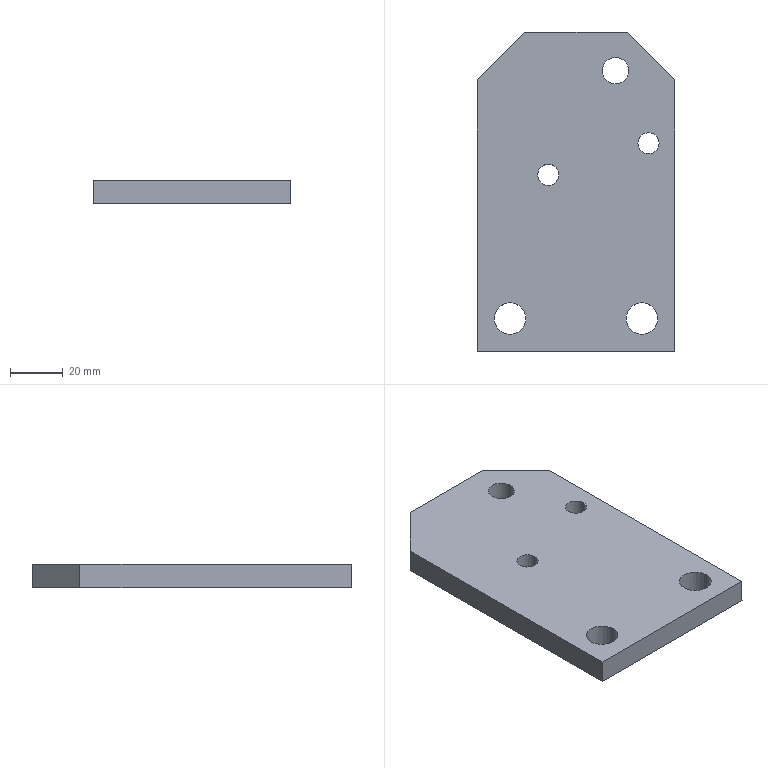Part | STEP file | J015-EBZ05-06-06-Part-1 | 1 solid | 18 faces | box 75 x 121 x 9 mm | volume 75112 mm3 | cylinder 10 | plane 8 | commonest cylinder face diameters 8 x4 12 x4 10 x2
STEP:
#1=CARTESIAN_POINT('',(6.5,13.5,0.));
#2=VERTEX_POINT('',#1);
#3=CARTESIAN_POINT('',(18.5,13.5,0.));
#4=VERTEX_POINT('',#3);
#5=CARTESIAN_POINT('',(12.5,13.5,0.));
#6=DIRECTION('',(0.,0.,-1.));
#7=DIRECTION('',(1.,0.,0.));
#8=AXIS2_PLACEMENT_3D('',#5,#6,#7);
#9=CIRCLE('',#8,6.);
#10=EDGE_CURVE('',#2,#4,#9,.T.);
#11=ORIENTED_EDGE('',*,*,#10,.F.);
#12=CARTESIAN_POINT('',(6.5,13.5,-9.));
#13=VERTEX_POINT('',#12);
#14=CARTESIAN_POINT('',(6.5,13.5,0.));
#15=DIRECTION('',(0.,0.,-1.));
#16=VECTOR('',#15,1000.);
#17=LINE('',#14,#16);
#18=EDGE_CURVE('',#2,#13,#17,.T.);
#19=ORIENTED_EDGE('',*,*,#18,.T.);
#20=CARTESIAN_POINT('',(18.5,13.5,-9.));
#21=VERTEX_POINT('',#20);
#22=CARTESIAN_POINT('',(12.5,13.5,-9.));
#23=DIRECTION('',(0.,0.,1.));
#24=DIRECTION('',(-1.,0.,0.));
#25=AXIS2_PLACEMENT_3D('',#22,#23,#24);
#26=CIRCLE('',#25,6.);
#27=EDGE_CURVE('',#21,#13,#26,.T.);
#28=ORIENTED_EDGE('',*,*,#27,.F.);
#29=CARTESIAN_POINT('',(18.5,13.5,0.));
#30=DIRECTION('',(0.,0.,-1.));
#31=VECTOR('',#30,1000.);
#32=LINE('',#29,#31);
#33=EDGE_CURVE('',#4,#21,#32,.T.);
#34=ORIENTED_EDGE('',*,*,#33,.F.);
#35=EDGE_LOOP('',(#11,#19,#28,#34));
#36=FACE_OUTER_BOUND('',#35,.T.);
#37=CARTESIAN_POINT('',(12.5,13.5,0.));
#38=DIRECTION('',(0.,0.,-1.));
#39=DIRECTION('',(1.,0.,0.));
#40=AXIS2_PLACEMENT_3D('',#37,#38,#39);
#41=CYLINDRICAL_SURFACE('',#40,6.);
#42=ADVANCED_FACE('',(#36),#41,.F.);
#43=CARTESIAN_POINT('',(56.5,13.5,0.));
#44=VERTEX_POINT('',#43);
#45=CARTESIAN_POINT('',(68.5,13.5,0.));
#46=VERTEX_POINT('',#45);
#47=CARTESIAN_POINT('',(62.5,13.5,0.));
#48=DIRECTION('',(0.,0.,-1.));
#49=DIRECTION('',(1.,0.,0.));
#50=AXIS2_PLACEMENT_3D('',#47,#48,#49);
#51=CIRCLE('',#50,6.);
#52=EDGE_CURVE('',#44,#46,#51,.T.);
#53=ORIENTED_EDGE('',*,*,#52,.F.);
#54=CARTESIAN_POINT('',(56.5,13.5,-9.));
#55=VERTEX_POINT('',#54);
#56=CARTESIAN_POINT('',(56.5,13.5,0.));
#57=DIRECTION('',(0.,0.,-1.));
#58=VECTOR('',#57,1000.);
#59=LINE('',#56,#58);
#60=EDGE_CURVE('',#44,#55,#59,.T.);
#61=ORIENTED_EDGE('',*,*,#60,.T.);
#62=CARTESIAN_POINT('',(68.5,13.5,-9.));
#63=VERTEX_POINT('',#62);
#64=CARTESIAN_POINT('',(62.5,13.5,-9.));
#65=DIRECTION('',(0.,0.,1.));
#66=DIRECTION('',(-1.,0.,0.));
#67=AXIS2_PLACEMENT_3D('',#64,#65,#66);
#68=CIRCLE('',#67,6.);
#69=EDGE_CURVE('',#63,#55,#68,.T.);
#70=ORIENTED_EDGE('',*,*,#69,.F.);
#71=CARTESIAN_POINT('',(68.5,13.5,0.));
#72=DIRECTION('',(0.,0.,-1.));
#73=VECTOR('',#72,1000.);
#74=LINE('',#71,#73);
#75=EDGE_CURVE('',#46,#63,#74,.T.);
#76=ORIENTED_EDGE('',*,*,#75,.F.);
#77=EDGE_LOOP('',(#53,#61,#70,#76));
#78=FACE_OUTER_BOUND('',#77,.T.);
#79=CARTESIAN_POINT('',(62.5,13.5,0.));
#80=DIRECTION('',(0.,0.,-1.));
#81=DIRECTION('',(1.,0.,0.));
#82=AXIS2_PLACEMENT_3D('',#79,#80,#81);
#83=CYLINDRICAL_SURFACE('',#82,6.);
#84=ADVANCED_FACE('',(#78),#83,.F.);
#85=CARTESIAN_POINT('',(69.,80.,0.));
#86=VERTEX_POINT('',#85);
#87=CARTESIAN_POINT('',(61.,80.,0.));
#88=VERTEX_POINT('',#87);
#89=CARTESIAN_POINT('',(65.,80.,0.));
#90=DIRECTION('',(0.,0.,1.));
#91=DIRECTION('',(-1.,0.,0.));
#92=AXIS2_PLACEMENT_3D('',#89,#90,#91);
#93=CIRCLE('',#92,4.);
#94=EDGE_CURVE('',#86,#88,#93,.T.);
#95=ORIENTED_EDGE('',*,*,#94,.T.);
#96=CARTESIAN_POINT('',(61.,80.,-9.));
#97=VERTEX_POINT('',#96);
#98=CARTESIAN_POINT('',(61.,80.,0.2));
#99=DIRECTION('',(0.,0.,-1.));
#100=VECTOR('',#99,1000.);
#101=LINE('',#98,#100);
#102=EDGE_CURVE('',#88,#97,#101,.T.);
#103=ORIENTED_EDGE('',*,*,#102,.T.);
#104=CARTESIAN_POINT('',(69.,80.,-9.));
#105=VERTEX_POINT('',#104);
#106=CARTESIAN_POINT('',(65.,80.,-9.));
#107=DIRECTION('',(0.,0.,1.));
#108=DIRECTION('',(-1.,0.,0.));
#109=AXIS2_PLACEMENT_3D('',#106,#107,#108);
#110=CIRCLE('',#109,4.);
#111=EDGE_CURVE('',#105,#97,#110,.T.);
#112=ORIENTED_EDGE('',*,*,#111,.F.);
#113=CARTESIAN_POINT('',(69.,80.,0.2));
#114=DIRECTION('',(0.,0.,-1.));
#115=VECTOR('',#114,1000.);
#116=LINE('',#113,#115);
#117=EDGE_CURVE('',#86,#105,#116,.T.);
#118=ORIENTED_EDGE('',*,*,#117,.F.);
#119=EDGE_LOOP('',(#95,#103,#112,#118));
#120=FACE_OUTER_BOUND('',#119,.T.);
#121=CARTESIAN_POINT('',(65.,80.,0.2));
#122=DIRECTION('',(0.,0.,-1.));
#123=DIRECTION('',(1.,0.,0.));
#124=AXIS2_PLACEMENT_3D('',#121,#122,#123);
#125=CYLINDRICAL_SURFACE('',#124,4.);
#126=ADVANCED_FACE('',(#120),#125,.F.);
#127=CARTESIAN_POINT('',(23.,68.,0.));
#128=VERTEX_POINT('',#127);
#129=CARTESIAN_POINT('',(31.,68.,0.));
#130=VERTEX_POINT('',#129);
#131=CARTESIAN_POINT('',(27.,68.,0.));
#132=DIRECTION('',(0.,0.,-1.));
#133=DIRECTION('',(1.,0.,0.));
#134=AXIS2_PLACEMENT_3D('',#131,#132,#133);
#135=CIRCLE('',#134,4.);
#136=EDGE_CURVE('',#128,#130,#135,.T.);
#137=ORIENTED_EDGE('',*,*,#136,.F.);
#138=CARTESIAN_POINT('',(23.,68.,-9.));
#139=VERTEX_POINT('',#138);
#140=CARTESIAN_POINT('',(23.,68.,0.));
#141=DIRECTION('',(0.,0.,-1.));
#142=VECTOR('',#141,1000.);
#143=LINE('',#140,#142);
#144=EDGE_CURVE('',#128,#139,#143,.T.);
#145=ORIENTED_EDGE('',*,*,#144,.T.);
#146=CARTESIAN_POINT('',(31.,68.,-9.));
#147=VERTEX_POINT('',#146);
#148=CARTESIAN_POINT('',(27.,68.,-9.));
#149=DIRECTION('',(0.,0.,1.));
#150=DIRECTION('',(-1.,0.,0.));
#151=AXIS2_PLACEMENT_3D('',#148,#149,#150);
#152=CIRCLE('',#151,4.);
#153=EDGE_CURVE('',#147,#139,#152,.T.);
#154=ORIENTED_EDGE('',*,*,#153,.F.);
#155=CARTESIAN_POINT('',(31.,68.,0.));
#156=DIRECTION('',(0.,0.,-1.));
#157=VECTOR('',#156,1000.);
#158=LINE('',#155,#157);
#159=EDGE_CURVE('',#130,#147,#158,.T.);
#160=ORIENTED_EDGE('',*,*,#159,.F.);
#161=EDGE_LOOP('',(#137,#145,#154,#160));
#162=FACE_OUTER_BOUND('',#161,.T.);
#163=CARTESIAN_POINT('',(27.,68.,0.));
#164=DIRECTION('',(0.,0.,-1.));
#165=DIRECTION('',(1.,0.,0.));
#166=AXIS2_PLACEMENT_3D('',#163,#164,#165);
#167=CYLINDRICAL_SURFACE('',#166,4.);
#168=ADVANCED_FACE('',(#162),#167,.F.);
#169=CARTESIAN_POINT('',(57.5,107.5,0.));
#170=VERTEX_POINT('',#169);
#171=CARTESIAN_POINT('',(47.5,107.5,0.));
#172=VERTEX_POINT('',#171);
#173=CARTESIAN_POINT('',(52.5,107.5,0.));
#174=DIRECTION('',(0.,0.,1.));
#175=DIRECTION('',(-1.,0.,0.));
#176=AXIS2_PLACEMENT_3D('',#173,#174,#175);
#177=CIRCLE('',#176,5.);
#178=EDGE_CURVE('',#170,#172,#177,.T.);
#179=ORIENTED_EDGE('',*,*,#178,.T.);
#180=CARTESIAN_POINT('',(47.5,107.5,-9.));
#181=VERTEX_POINT('',#180);
#182=CARTESIAN_POINT('',(47.5,107.5,-9.));
#183=DIRECTION('',(0.,0.,-1.));
#184=VECTOR('',#183,1000.);
#185=LINE('',#182,#184);
#186=EDGE_CURVE('',#172,#181,#185,.T.);
#187=ORIENTED_EDGE('',*,*,#186,.T.);
#188=CARTESIAN_POINT('',(57.5,107.5,-9.));
#189=VERTEX_POINT('',#188);
#190=CARTESIAN_POINT('',(52.5,107.5,-9.));
#191=DIRECTION('',(0.,0.,-1.));
#192=DIRECTION('',(1.,0.,0.));
#193=AXIS2_PLACEMENT_3D('',#190,#191,#192);
#194=CIRCLE('',#193,5.);
#195=EDGE_CURVE('',#181,#189,#194,.T.);
#196=ORIENTED_EDGE('',*,*,#195,.T.);
#197=CARTESIAN_POINT('',(57.5,107.5,-9.));
#198=DIRECTION('',(0.,0.,-1.));
#199=VECTOR('',#198,1000.);
#200=LINE('',#197,#199);
#201=EDGE_CURVE('',#170,#189,#200,.T.);
#202=ORIENTED_EDGE('',*,*,#201,.F.);
#203=EDGE_LOOP('',(#179,#187,#196,#202));
#204=FACE_OUTER_BOUND('',#203,.T.);
#205=CARTESIAN_POINT('',(52.5,107.5,-9.));
#206=DIRECTION('',(0.,0.,-1.));
#207=DIRECTION('',(1.,0.,0.));
#208=AXIS2_PLACEMENT_3D('',#205,#206,#207);
#209=CYLINDRICAL_SURFACE('',#208,5.);
#210=ADVANCED_FACE('',(#204),#209,.F.);
#211=CARTESIAN_POINT('',(0.,104.,0.));
#212=VERTEX_POINT('',#211);
#213=CARTESIAN_POINT('',(0.,1.,0.));
#214=VERTEX_POINT('',#213);
#215=CARTESIAN_POINT('',(0.,95.5,0.));
#216=DIRECTION('',(0.,-1.,0.));
#217=VECTOR('',#216,1000.);
#218=LINE('',#215,#217);
#219=EDGE_CURVE('',#212,#214,#218,.T.);
#220=ORIENTED_EDGE('',*,*,#219,.F.);
#221=CARTESIAN_POINT('',(0.,104.,-9.));
#222=VERTEX_POINT('',#221);
#223=CARTESIAN_POINT('',(0.,104.,-41.114));
#224=DIRECTION('',(0.,0.,-1.));
#225=VECTOR('',#224,1000.);
#226=LINE('',#223,#225);
#227=EDGE_CURVE('',#212,#222,#226,.T.);
#228=ORIENTED_EDGE('',*,*,#227,.T.);
#229=CARTESIAN_POINT('',(0.,1.,-9.));
#230=VERTEX_POINT('',#229);
#231=CARTESIAN_POINT('',(0.,51.5,-9.));
#232=DIRECTION('',(0.,1.,0.));
#233=VECTOR('',#232,1000.);
#234=LINE('',#231,#233);
#235=EDGE_CURVE('',#230,#222,#234,.T.);
#236=ORIENTED_EDGE('',*,*,#235,.F.);
#237=CARTESIAN_POINT('',(0.,1.,-14.));
#238=DIRECTION('',(0.,0.,1.));
#239=VECTOR('',#238,1000.);
#240=LINE('',#237,#239);
#241=EDGE_CURVE('',#230,#214,#240,.T.);
#242=ORIENTED_EDGE('',*,*,#241,.T.);
#243=EDGE_LOOP('',(#220,#228,#236,#242));
#244=FACE_OUTER_BOUND('',#243,.T.);
#245=CARTESIAN_POINT('',(0.,38.386,-41.114));
#246=DIRECTION('',(-1.,0.,0.));
#247=DIRECTION('',(0.,1.,0.));
#248=AXIS2_PLACEMENT_3D('',#245,#246,#247);
#249=PLANE('',#248);
#250=ADVANCED_FACE('',(#244),#249,.T.);
#251=CARTESIAN_POINT('',(75.,1.,-9.));
#252=VERTEX_POINT('',#251);
#253=CARTESIAN_POINT('',(75.,1.,0.));
#254=VERTEX_POINT('',#253);
#255=CARTESIAN_POINT('',(75.,1.,-14.));
#256=DIRECTION('',(0.,0.,1.));
#257=VECTOR('',#256,1000.);
#258=LINE('',#255,#257);
#259=EDGE_CURVE('',#252,#254,#258,.T.);
#260=ORIENTED_EDGE('',*,*,#259,.T.);
#261=CARTESIAN_POINT('',(95.016,1.,0.));
#262=DIRECTION('',(-1.,0.,0.));
#263=VECTOR('',#262,1000.);
#264=LINE('',#261,#263);
#265=EDGE_CURVE('',#254,#214,#264,.T.);
#266=ORIENTED_EDGE('',*,*,#265,.T.);
#267=ORIENTED_EDGE('',*,*,#241,.F.);
#268=CARTESIAN_POINT('',(75.,1.,-9.));
#269=DIRECTION('',(-1.,0.,0.));
#270=VECTOR('',#269,1000.);
#271=LINE('',#268,#270);
#272=EDGE_CURVE('',#252,#230,#271,.T.);
#273=ORIENTED_EDGE('',*,*,#272,.F.);
#274=EDGE_LOOP('',(#260,#266,#267,#273));
#275=FACE_OUTER_BOUND('',#274,.T.);
#276=CARTESIAN_POINT('',(95.016,1.,-63.516));
#277=DIRECTION('',(0.,-1.,0.));
#278=DIRECTION('',(-1.,0.,0.));
#279=AXIS2_PLACEMENT_3D('',#276,#277,#278);
#280=PLANE('',#279);
#281=ADVANCED_FACE('',(#275),#280,.T.);
#282=CARTESIAN_POINT('',(75.,104.,-9.));
#283=VERTEX_POINT('',#282);
#284=CARTESIAN_POINT('',(75.,110.5,-9.));
#285=DIRECTION('',(0.,-1.,0.));
#286=VECTOR('',#285,1000.);
#287=LINE('',#284,#286);
#288=EDGE_CURVE('',#283,#252,#287,.T.);
#289=ORIENTED_EDGE('',*,*,#288,.F.);
#290=CARTESIAN_POINT('',(75.,104.,0.));
#291=VERTEX_POINT('',#290);
#292=CARTESIAN_POINT('',(75.,104.,-51.848));
#293=DIRECTION('',(0.,0.,1.));
#294=VECTOR('',#293,1000.);
#295=LINE('',#292,#294);
#296=EDGE_CURVE('',#283,#291,#295,.T.);
#297=ORIENTED_EDGE('',*,*,#296,.T.);
#298=CARTESIAN_POINT('',(75.,110.5,0.));
#299=DIRECTION('',(0.,-1.,0.));
#300=VECTOR('',#299,1000.);
#301=LINE('',#298,#300);
#302=EDGE_CURVE('',#291,#254,#301,.T.);
#303=ORIENTED_EDGE('',*,*,#302,.T.);
#304=ORIENTED_EDGE('',*,*,#259,.F.);
#305=EDGE_LOOP('',(#289,#297,#303,#304));
#306=FACE_OUTER_BOUND('',#305,.T.);
#307=CARTESIAN_POINT('',(75.,126.848,-51.848));
#308=DIRECTION('',(1.,0.,0.));
#309=DIRECTION('',(0.,-1.,0.));
#310=AXIS2_PLACEMENT_3D('',#307,#308,#309);
#311=PLANE('',#310);
#312=ADVANCED_FACE('',(#306),#311,.T.);
#313=ORIENTED_EDGE('',*,*,#27,.T.);
#314=CARTESIAN_POINT('',(12.5,13.5,-9.));
#315=DIRECTION('',(0.,0.,1.));
#316=DIRECTION('',(-1.,0.,0.));
#317=AXIS2_PLACEMENT_3D('',#314,#315,#316);
#318=CIRCLE('',#317,6.);
#319=EDGE_CURVE('',#13,#21,#318,.T.);
#320=ORIENTED_EDGE('',*,*,#319,.T.);
#321=EDGE_LOOP('',(#313,#320));
#322=FACE_BOUND('',#321,.T.);
#323=ORIENTED_EDGE('',*,*,#69,.T.);
#324=CARTESIAN_POINT('',(62.5,13.5,-9.));
#325=DIRECTION('',(0.,0.,1.));
#326=DIRECTION('',(-1.,0.,0.));
#327=AXIS2_PLACEMENT_3D('',#324,#325,#326);
#328=CIRCLE('',#327,6.);
#329=EDGE_CURVE('',#55,#63,#328,.T.);
#330=ORIENTED_EDGE('',*,*,#329,.T.);
#331=EDGE_LOOP('',(#323,#330));
#332=FACE_BOUND('',#331,.T.);
#333=ORIENTED_EDGE('',*,*,#111,.T.);
#334=CARTESIAN_POINT('',(65.,80.,-9.));
#335=DIRECTION('',(0.,0.,1.));
#336=DIRECTION('',(-1.,0.,0.));
#337=AXIS2_PLACEMENT_3D('',#334,#335,#336);
#338=CIRCLE('',#337,4.);
#339=EDGE_CURVE('',#97,#105,#338,.T.);
#340=ORIENTED_EDGE('',*,*,#339,.T.);
#341=EDGE_LOOP('',(#333,#340));
#342=FACE_BOUND('',#341,.T.);
#343=ORIENTED_EDGE('',*,*,#153,.T.);
#344=CARTESIAN_POINT('',(27.,68.,-9.));
#345=DIRECTION('',(0.,0.,1.));
#346=DIRECTION('',(-1.,0.,0.));
#347=AXIS2_PLACEMENT_3D('',#344,#345,#346);
#348=CIRCLE('',#347,4.);
#349=EDGE_CURVE('',#139,#147,#348,.T.);
#350=ORIENTED_EDGE('',*,*,#349,.T.);
#351=EDGE_LOOP('',(#343,#350));
#352=FACE_BOUND('',#351,.T.);
#353=CARTESIAN_POINT('',(52.5,107.5,-9.));
#354=DIRECTION('',(0.,0.,-1.));
#355=DIRECTION('',(1.,0.,0.));
#356=AXIS2_PLACEMENT_3D('',#353,#354,#355);
#357=CIRCLE('',#356,5.);
#358=EDGE_CURVE('',#189,#181,#357,.T.);
#359=ORIENTED_EDGE('',*,*,#358,.F.);
#360=ORIENTED_EDGE('',*,*,#195,.F.);
#361=EDGE_LOOP('',(#359,#360));
#362=FACE_BOUND('',#361,.T.);
#363=ORIENTED_EDGE('',*,*,#235,.T.);
#364=CARTESIAN_POINT('',(18.,122.,-9.));
#365=VERTEX_POINT('',#364);
#366=CARTESIAN_POINT('',(18.,122.,-9.));
#367=DIRECTION('',(0.7071,0.7071,0.));
#368=VECTOR('',#367,1000.);
#369=LINE('',#366,#368);
#370=EDGE_CURVE('',#222,#365,#369,.T.);
#371=ORIENTED_EDGE('',*,*,#370,.T.);
#372=CARTESIAN_POINT('',(57.,122.,-9.));
#373=VERTEX_POINT('',#372);
#374=CARTESIAN_POINT('',(25.,122.,-9.));
#375=DIRECTION('',(1.,0.,0.));
#376=VECTOR('',#375,1000.);
#377=LINE('',#374,#376);
#378=EDGE_CURVE('',#365,#373,#377,.T.);
#379=ORIENTED_EDGE('',*,*,#378,.T.);
#380=CARTESIAN_POINT('',(75.,104.,-9.));
#381=DIRECTION('',(0.7071,-0.7071,0.));
#382=VECTOR('',#381,1000.);
#383=LINE('',#380,#382);
#384=EDGE_CURVE('',#373,#283,#383,.T.);
#385=ORIENTED_EDGE('',*,*,#384,.T.);
#386=ORIENTED_EDGE('',*,*,#288,.T.);
#387=ORIENTED_EDGE('',*,*,#272,.T.);
#388=EDGE_LOOP('',(#363,#371,#379,#385,#386,#387));
#389=FACE_OUTER_BOUND('',#388,.T.);
#390=CARTESIAN_POINT('',(113.934,162.434,-9.));
#391=DIRECTION('',(0.,0.,1.));
#392=DIRECTION('',(0.,-1.,0.));
#393=AXIS2_PLACEMENT_3D('',#390,#391,#392);
#394=PLANE('',#393);
#395=ADVANCED_FACE('',(#322,#332,#342,#352,#362,#389),#394,.F.);
#396=ORIENTED_EDGE('',*,*,#378,.F.);
#397=CARTESIAN_POINT('',(18.,122.,0.));
#398=VERTEX_POINT('',#397);
#399=CARTESIAN_POINT('',(18.,122.,-38.784));
#400=DIRECTION('',(0.,0.,1.));
#401=VECTOR('',#400,1000.);
#402=LINE('',#399,#401);
#403=EDGE_CURVE('',#365,#398,#402,.T.);
#404=ORIENTED_EDGE('',*,*,#403,.T.);
#405=CARTESIAN_POINT('',(57.,122.,0.));
#406=VERTEX_POINT('',#405);
#407=CARTESIAN_POINT('',(25.,122.,0.));
#408=DIRECTION('',(1.,0.,0.));
#409=VECTOR('',#408,1000.);
#410=LINE('',#407,#409);
#411=EDGE_CURVE('',#398,#406,#410,.T.);
#412=ORIENTED_EDGE('',*,*,#411,.T.);
#413=CARTESIAN_POINT('',(57.,122.,-38.784));
#414=DIRECTION('',(0.,0.,-1.));
#415=VECTOR('',#414,1000.);
#416=LINE('',#413,#415);
#417=EDGE_CURVE('',#406,#373,#416,.T.);
#418=ORIENTED_EDGE('',*,*,#417,.T.);
#419=EDGE_LOOP('',(#396,#404,#412,#418));
#420=FACE_OUTER_BOUND('',#419,.T.);
#421=CARTESIAN_POINT('',(13.216,122.,-38.784));
#422=DIRECTION('',(0.,1.,0.));
#423=DIRECTION('',(1.,0.,0.));
#424=AXIS2_PLACEMENT_3D('',#421,#422,#423);
#425=PLANE('',#424);
#426=ADVANCED_FACE('',(#420),#425,.T.);
#427=CARTESIAN_POINT('',(12.5,13.5,0.));
#428=DIRECTION('',(0.,0.,-1.));
#429=DIRECTION('',(1.,0.,0.));
#430=AXIS2_PLACEMENT_3D('',#427,#428,#429);
#431=CIRCLE('',#430,6.);
#432=EDGE_CURVE('',#4,#2,#431,.T.);
#433=ORIENTED_EDGE('',*,*,#432,.T.);
#434=ORIENTED_EDGE('',*,*,#10,.T.);
#435=EDGE_LOOP('',(#433,#434));
#436=FACE_BOUND('',#435,.T.);
#437=CARTESIAN_POINT('',(62.5,13.5,0.));
#438=DIRECTION('',(0.,0.,-1.));
#439=DIRECTION('',(1.,0.,0.));
#440=AXIS2_PLACEMENT_3D('',#437,#438,#439);
#441=CIRCLE('',#440,6.);
#442=EDGE_CURVE('',#46,#44,#441,.T.);
#443=ORIENTED_EDGE('',*,*,#442,.T.);
#444=ORIENTED_EDGE('',*,*,#52,.T.);
#445=EDGE_LOOP('',(#443,#444));
#446=FACE_BOUND('',#445,.T.);
#447=ORIENTED_EDGE('',*,*,#94,.F.);
#448=CARTESIAN_POINT('',(65.,80.,0.));
#449=DIRECTION('',(0.,0.,1.));
#450=DIRECTION('',(-1.,0.,0.));
#451=AXIS2_PLACEMENT_3D('',#448,#449,#450);
#452=CIRCLE('',#451,4.);
#453=EDGE_CURVE('',#88,#86,#452,.T.);
#454=ORIENTED_EDGE('',*,*,#453,.F.);
#455=EDGE_LOOP('',(#447,#454));
#456=FACE_BOUND('',#455,.T.);
#457=CARTESIAN_POINT('',(27.,68.,0.));
#458=DIRECTION('',(0.,0.,-1.));
#459=DIRECTION('',(1.,0.,0.));
#460=AXIS2_PLACEMENT_3D('',#457,#458,#459);
#461=CIRCLE('',#460,4.);
#462=EDGE_CURVE('',#130,#128,#461,.T.);
#463=ORIENTED_EDGE('',*,*,#462,.T.);
#464=ORIENTED_EDGE('',*,*,#136,.T.);
#465=EDGE_LOOP('',(#463,#464));
#466=FACE_BOUND('',#465,.T.);
#467=ORIENTED_EDGE('',*,*,#178,.F.);
#468=CARTESIAN_POINT('',(52.5,107.5,0.));
#469=DIRECTION('',(0.,0.,1.));
#470=DIRECTION('',(-1.,0.,0.));
#471=AXIS2_PLACEMENT_3D('',#468,#469,#470);
#472=CIRCLE('',#471,5.);
#473=EDGE_CURVE('',#172,#170,#472,.T.);
#474=ORIENTED_EDGE('',*,*,#473,.F.);
#475=EDGE_LOOP('',(#467,#474));
#476=FACE_BOUND('',#475,.T.);
#477=ORIENTED_EDGE('',*,*,#411,.F.);
#478=CARTESIAN_POINT('',(83.819,187.819,0.));
#479=DIRECTION('',(-0.7071,-0.7071,0.));
#480=VECTOR('',#479,1000.);
#481=LINE('',#478,#480);
#482=EDGE_CURVE('',#398,#212,#481,.T.);
#483=ORIENTED_EDGE('',*,*,#482,.T.);
#484=ORIENTED_EDGE('',*,*,#219,.T.);
#485=ORIENTED_EDGE('',*,*,#265,.F.);
#486=ORIENTED_EDGE('',*,*,#302,.F.);
#487=CARTESIAN_POINT('',(62.75,116.25,0.));
#488=DIRECTION('',(-0.7071,0.7071,0.));
#489=VECTOR('',#488,1000.);
#490=LINE('',#487,#489);
#491=EDGE_CURVE('',#291,#406,#490,.T.);
#492=ORIENTED_EDGE('',*,*,#491,.T.);
#493=EDGE_LOOP('',(#477,#483,#484,#485,#486,#492));
#494=FACE_OUTER_BOUND('',#493,.T.);
#495=CARTESIAN_POINT('',(109.069,162.569,0.));
#496=DIRECTION('',(0.,0.,1.));
#497=DIRECTION('',(0.,-1.,0.));
#498=AXIS2_PLACEMENT_3D('',#495,#496,#497);
#499=PLANE('',#498);
#500=ADVANCED_FACE('',(#436,#446,#456,#466,#476,#494),#499,.T.);
#501=ORIENTED_EDGE('',*,*,#186,.F.);
#502=ORIENTED_EDGE('',*,*,#473,.T.);
#503=ORIENTED_EDGE('',*,*,#201,.T.);
#504=ORIENTED_EDGE('',*,*,#358,.T.);
#505=EDGE_LOOP('',(#501,#502,#503,#504));
#506=FACE_OUTER_BOUND('',#505,.T.);
#507=CARTESIAN_POINT('',(52.5,107.5,-9.));
#508=DIRECTION('',(0.,0.,-1.));
#509=DIRECTION('',(1.,0.,0.));
#510=AXIS2_PLACEMENT_3D('',#507,#508,#509);
#511=CYLINDRICAL_SURFACE('',#510,5.);
#512=ADVANCED_FACE('',(#506),#511,.F.);
#513=ORIENTED_EDGE('',*,*,#384,.F.);
#514=ORIENTED_EDGE('',*,*,#417,.F.);
#515=ORIENTED_EDGE('',*,*,#491,.F.);
#516=ORIENTED_EDGE('',*,*,#296,.F.);
#517=EDGE_LOOP('',(#513,#514,#515,#516));
#518=FACE_OUTER_BOUND('',#517,.T.);
#519=CARTESIAN_POINT('',(75.,104.,-51.848));
#520=DIRECTION('',(-0.7071,-0.7071,0.));
#521=DIRECTION('',(0.,0.,1.));
#522=AXIS2_PLACEMENT_3D('',#519,#520,#521);
#523=PLANE('',#522);
#524=ADVANCED_FACE('',(#518),#523,.F.);
#525=ORIENTED_EDGE('',*,*,#144,.F.);
#526=ORIENTED_EDGE('',*,*,#462,.F.);
#527=ORIENTED_EDGE('',*,*,#159,.T.);
#528=ORIENTED_EDGE('',*,*,#349,.F.);
#529=EDGE_LOOP('',(#525,#526,#527,#528));
#530=FACE_OUTER_BOUND('',#529,.T.);
#531=CARTESIAN_POINT('',(27.,68.,0.));
#532=DIRECTION('',(0.,0.,-1.));
#533=DIRECTION('',(1.,0.,0.));
#534=AXIS2_PLACEMENT_3D('',#531,#532,#533);
#535=CYLINDRICAL_SURFACE('',#534,4.);
#536=ADVANCED_FACE('',(#530),#535,.F.);
#537=ORIENTED_EDGE('',*,*,#102,.F.);
#538=ORIENTED_EDGE('',*,*,#453,.T.);
#539=ORIENTED_EDGE('',*,*,#117,.T.);
#540=ORIENTED_EDGE('',*,*,#339,.F.);
#541=EDGE_LOOP('',(#537,#538,#539,#540));
#542=FACE_OUTER_BOUND('',#541,.T.);
#543=CARTESIAN_POINT('',(65.,80.,0.2));
#544=DIRECTION('',(0.,0.,-1.));
#545=DIRECTION('',(1.,0.,0.));
#546=AXIS2_PLACEMENT_3D('',#543,#544,#545);
#547=CYLINDRICAL_SURFACE('',#546,4.);
#548=ADVANCED_FACE('',(#542),#547,.F.);
#549=ORIENTED_EDGE('',*,*,#370,.F.);
#550=ORIENTED_EDGE('',*,*,#227,.F.);
#551=ORIENTED_EDGE('',*,*,#482,.F.);
#552=ORIENTED_EDGE('',*,*,#403,.F.);
#553=EDGE_LOOP('',(#549,#550,#551,#552));
#554=FACE_OUTER_BOUND('',#553,.T.);
#555=CARTESIAN_POINT('',(18.,122.,-38.784));
#556=DIRECTION('',(0.7071,-0.7071,0.));
#557=DIRECTION('',(0.,0.,1.));
#558=AXIS2_PLACEMENT_3D('',#555,#556,#557);
#559=PLANE('',#558);
#560=ADVANCED_FACE('',(#554),#559,.F.);
#561=ORIENTED_EDGE('',*,*,#60,.F.);
#562=ORIENTED_EDGE('',*,*,#442,.F.);
#563=ORIENTED_EDGE('',*,*,#75,.T.);
#564=ORIENTED_EDGE('',*,*,#329,.F.);
#565=EDGE_LOOP('',(#561,#562,#563,#564));
#566=FACE_OUTER_BOUND('',#565,.T.);
#567=CARTESIAN_POINT('',(62.5,13.5,0.));
#568=DIRECTION('',(0.,0.,-1.));
#569=DIRECTION('',(1.,0.,0.));
#570=AXIS2_PLACEMENT_3D('',#567,#568,#569);
#571=CYLINDRICAL_SURFACE('',#570,6.);
#572=ADVANCED_FACE('',(#566),#571,.F.);
#573=ORIENTED_EDGE('',*,*,#18,.F.);
#574=ORIENTED_EDGE('',*,*,#432,.F.);
#575=ORIENTED_EDGE('',*,*,#33,.T.);
#576=ORIENTED_EDGE('',*,*,#319,.F.);
#577=EDGE_LOOP('',(#573,#574,#575,#576));
#578=FACE_OUTER_BOUND('',#577,.T.);
#579=CARTESIAN_POINT('',(12.5,13.5,0.));
#580=DIRECTION('',(0.,0.,-1.));
#581=DIRECTION('',(1.,0.,0.));
#582=AXIS2_PLACEMENT_3D('',#579,#580,#581);
#583=CYLINDRICAL_SURFACE('',#582,6.);
#584=ADVANCED_FACE('',(#578),#583,.F.);
#585=CLOSED_SHELL('',(#42,#84,#126,#168,#210,#250,#281,#312,#395,#426,#500,#512,#524,#536,#548,#560,#572,#584));
#586=MANIFOLD_SOLID_BREP('',#585);
#587=CARTESIAN_POINT('',(0.,0.,0.));
#588=DIRECTION('',(0.,0.,1.));
#589=DIRECTION('',(1.,0.,0.));
#590=AXIS2_PLACEMENT_3D('',#587,#588,#589);
#591=(LENGTH_UNIT()NAMED_UNIT(*)SI_UNIT(.MILLI.,.METRE.));
#592=UNCERTAINTY_MEASURE_WITH_UNIT(LENGTH_MEASURE(0.00001),#591,'','');
#593=(NAMED_UNIT(*)PLANE_ANGLE_UNIT()SI_UNIT($,.RADIAN.));
#594=(NAMED_UNIT(*)SI_UNIT($,.STERADIAN.)SOLID_ANGLE_UNIT());
#595=(GEOMETRIC_REPRESENTATION_CONTEXT(3)GLOBAL_UNCERTAINTY_ASSIGNED_CONTEXT((#592))GLOBAL_UNIT_ASSIGNED_CONTEXT((#591,#593,#594))REPRESENTATION_CONTEXT('',''));
#596=ADVANCED_BREP_SHAPE_REPRESENTATION('',(#586,#590),#595);